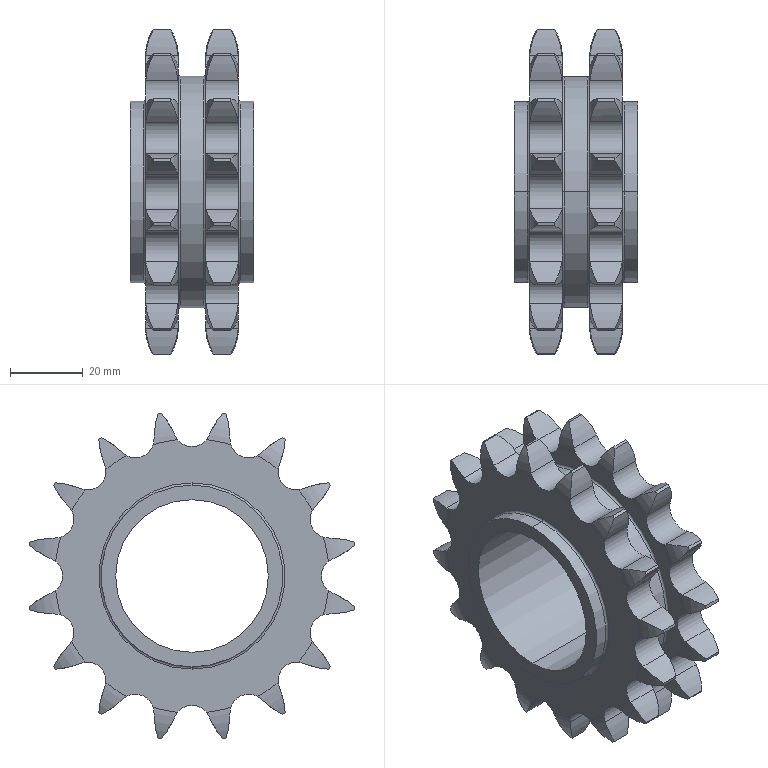Part | STEP file | short pitch roller chain wheel_d_iso_Chain wheel ISO - 16Z 10B-2 --16SC50H34L42.0N | 1 solid | 224 faces | box 34.001 x 89.463 x 89.463 mm | volume 79108 mm3 | cylinder 146 | torus 72 | plane 6 | commonest cylinder face diameters 43.891 x64 10.262 x42 91.056 x32 50 x4 42 x2 63.73 x2